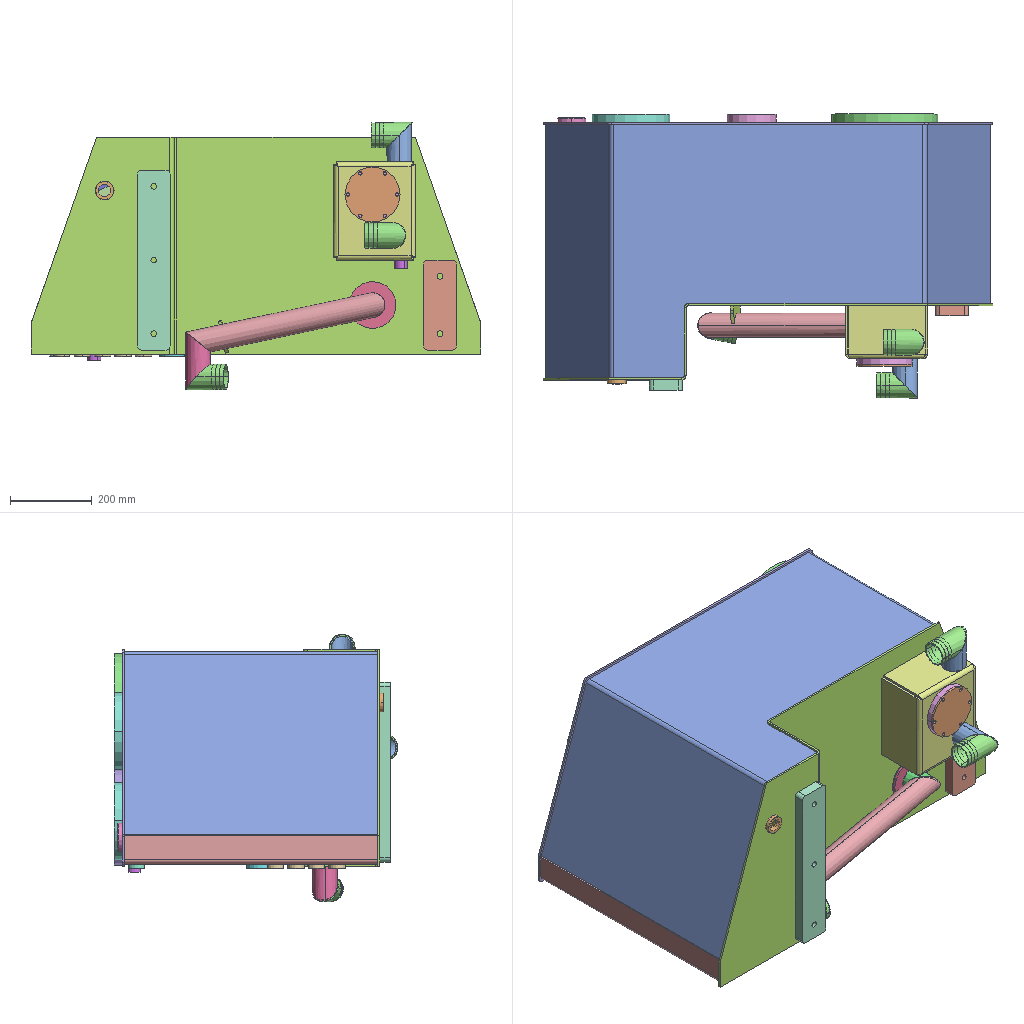Assembly | SolidWorks | 33 different items | 45 placed | box 1100 x 694 x 654 mm
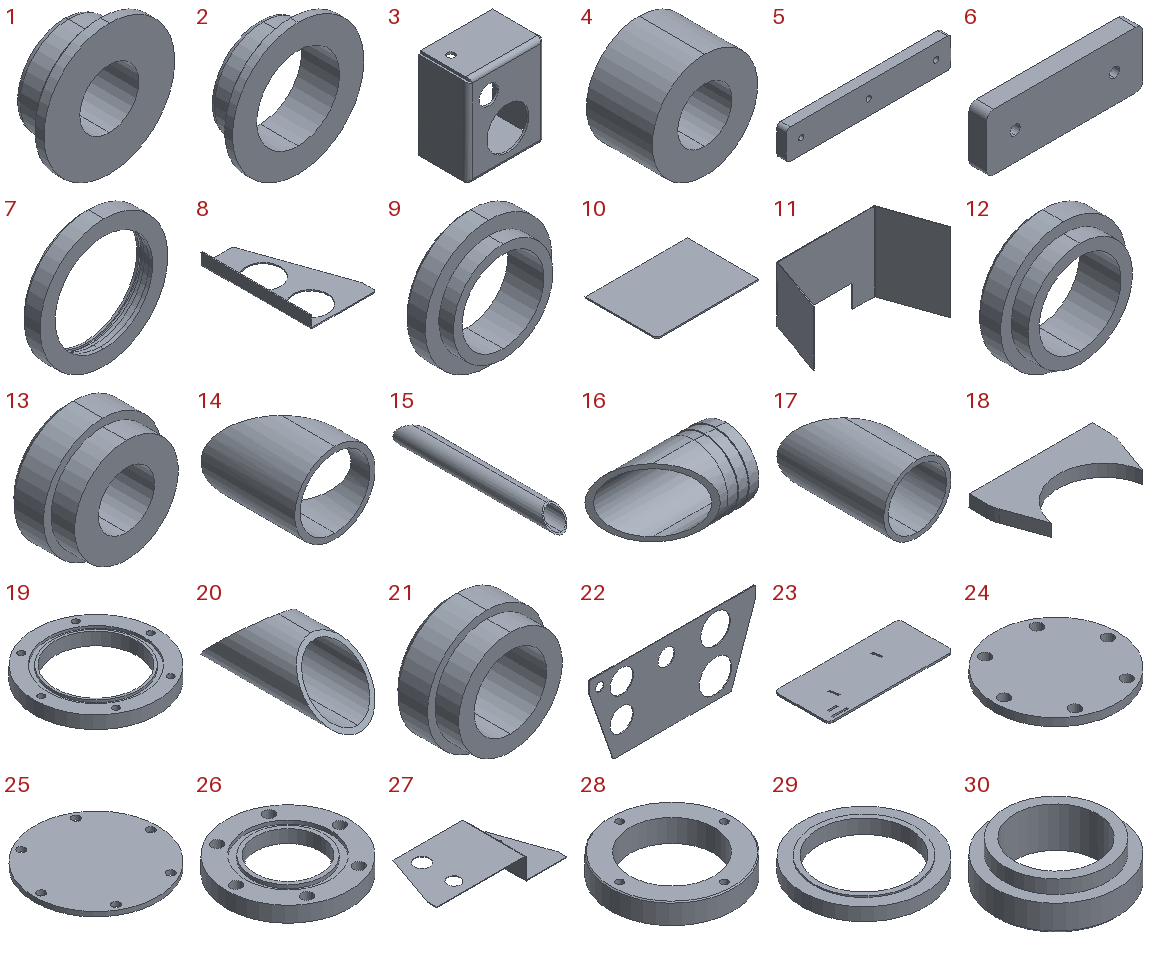Parts list (item | quantity | size | volume | features):
1 | x1 | 115 x 39 x 115 mm | 186319 mm3 | features Chamfer 1, Revolution 1
2 | x1 | 135 x 39 x 135 mm | 150743 mm3 | features Chamfer 1, Revolution 1
3 | x1 | 200 x 130 x 240 mm | 676018 mm3 | features ICE 5, Cut 1, EdgeFlange 1, FlatPattern 1, SMBaseFlange 1, SheetMetal 1, UnFold 1
4 | x2 | 32 x 20 x 32 mm | 11591 mm3 | features Chamfer 1, Extrusion 1, HoleWzd 1
5 | x1 | 440 x 25 x 80 mm | 866309 mm3 | features Fillet 1, FlatPattern 1, HoleWzd 1, LPattern 1, SMBaseFlange 1, SheetMetal 1
6 | x1 | 220 x 25 x 80 mm | 430157 mm3 | features Fillet 1, FlatPattern 1, HoleWzd 1, LPattern 1, SMBaseFlange 1, SheetMetal 1
7 | x2 | 170 x 26 x 170 mm | 194901 mm3 | features Revolution 1
8 | x1 | 305 x 510 x 58 mm | 526681 mm3 | features EdgeFlange 1, FlatPattern 1, ICE 1, SMBaseFlange 1, SheetMetal 1, UnFold 1
9 | x1 | 70 x 20 x 70 mm | 32594 mm3 | features Chamfer 1, HoleWzd 1, Revolution 1
10 | x2 | 400 x 280 x 5 mm | 559750 mm3 | features Chamfer 1, FlatPattern 1, ICE 1, LPattern 1, SMBaseFlange 1, SheetMetal 1
11 | x1 | 1088 x 449.658 x 620 mm | 4342657 mm3 | features Fillet 2, Cut 1, FlatPattern 1, SMBaseFlange 1, SheetMetal 1, UnFold 1
12 | x1 | 60 x 20 x 60 mm | 25069 mm3 | features Chamfer 1, HoleWzd 1, Revolution 1
13 | x6 | 40 x 20 x 40 mm | 16863 mm3 | features Chamfer 1, HoleWzd 1, Revolution 1
14 | x1 | 60 x 70 x 60 mm | 28148 mm3 | features Extrusion 1, ICE 1
15 | x1 | 60 x 490 x 60 mm | 306614 mm3 | features ICE 2, Extrusion 1
16 | x3 | 100 x 63 x 63 mm | 47848 mm3 | features ICE 1, Revolution 1
17 | x2 | 60 x 95 x 60 mm | 45740 mm3 | features Extrusion 1, ICE 1
18 | x1 | 80 x 43.435 x 8 mm | 16306 mm3 | features Fillet 1, FlatPattern 1, SMBaseFlange 1, SheetMetal 1
19 | x1 | 135 x 135 x 14 mm | 104256 mm3 | features ICE 2, CirPattern 1, FlatPattern 1, HoleWzd 1, SMBaseFlange 1, SheetMetal 1
20 | x1 | 60 x 140 x 60 mm | 60313 mm3 | features BaseBody 1
21 | x1 | 40 x 20 x 40 mm | 13105 mm3 | features Chamfer 1, HoleWzd 1, Revolution 1
22 | x1 | 1100 x 5 x 530 mm | 1971755 mm3 | features Fillet 1, FlatPattern 1, ICE 1, SMBaseFlange 1, SheetMetal 1
23 | x1 | 550 x 240 x 8 mm | 1041413 mm3 | features FlatPattern 1, SMBaseFlange 1, SheetMetal 1
24 | x1 | 95 x 95 x 6 mm | 40486 mm3 | features FlatPattern 1, SMBaseFlange 1, SheetMetal 1
25 | x1 | 135 x 135 x 5 mm | 69867 mm3 | features CirPattern 1, FlatPattern 1, ICE 1, SMBaseFlange 1, SheetMetal 1
26 | x1 | 95 x 95 x 12 mm | 53096 mm3 | features ICE 2, CirPattern 1, FlatPattern 1, HoleWzd 1, SMBaseFlange 1, SheetMetal 1
27 | x1 | 1100 x 530 x 187 mm | 2899151 mm3 | features Cut 2, EdgeFlange 2, ICE 2, FlatPattern 1, SMBaseFlange 1, SheetMetal 1, UnFold 1
28 | x1 | 120 x 120 x 22 mm | 125864 mm3 | features Chamfer 1, CirPattern 1, FlatPattern 1, HoleWzd 1, ICE 1, SMBaseFlange 1, SheetMetal 1
29 | x2 | 190 x 190 x 22 mm | 258295 mm3 | features ICE 2, 3DProfileFeature 1, CirPattern 1, FlatPattern 1, HoleWzd 1, SMBaseFlange 1, SheetMetal 1
30 | x1 | 46 x 46 x 15 mm | 11079 mm3 | features ICE 3, Chamfer 1, Extrusion 1, HoleWzd 1
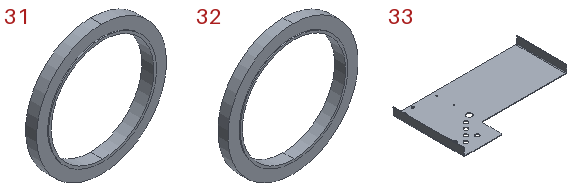31 | x1 | 235 x 22 x 235 mm | 321081 mm3 | features CirPattern 1, FlatPattern 1, HoleWzd 1, ICE 1, SMBaseFlange 1, SheetMetal 1
32 | x1 | 260 x 22 x 260 mm | 392882 mm3 | features CirPattern 1, FlatPattern 1, HoleWzd 1, ICE 1, SMBaseFlange 1, SheetMetal 1
33 | x1 | 1090 x 620 x 70 mm | 2975093 mm3 | features Cut 3, Fillet 2, EdgeFlange 1, FlatPattern 1, ICE 1, SMBaseFlange 1, SheetMetal 1, UnFold 1
Mates (type | each side: item.copy, entity, surface, feature):
Coincident | 33.1 face plane Edge-Flange1 | 11.1 face plane Base-Flange1
Coincident | 33.1 face plane Cut-Extrude1 | 27.1 face plane Base-Flange1
Parallel | 33.1 face plane Edge-Flange1 | 31.1 plane
Parallel | 32.1 plane | 33.1 face plane Edge-Flange1
Concentric | 27.1 face cylinder Cut-Extrude4 | 2.1 face cylinder Revolve1
Coincident | 27.1 face plane Base-Flange1 | 2.1 face plane Revolve1
Coincident | 27.1 face plane Base-Flange1 | 3.1 face plane Edge-Flange1
DistanceDim | 3.1 face plane Edge-Flange1 | 27.1 face plane Base-Flange1 | 2 times
Coincident | 27.1 face plane Edge-Flange2 | 5.1 face plane Base-Flange1
DistanceDim | 5.1 face plane Base-Flange1 | 27.1 face plane Edge-Flange2
DistanceDim | 5.1 face plane Base-Flange1 | 27.1 face plane Edge-Flange1
Coincident | 27.1 face plane Base-Flange1 | 6.1 face plane Base-Flange1
DistanceDim | 6.1 face plane Base-Flange1 | 27.1 face plane Base-Flange1 | 2 times
Parallel | 33.1 face plane Base-Flange1 | 28.1 plane
Coincident | 27.1 face plane Edge-Flange2 | 30.1 face plane Boss-Extrude2
Concentric | 27.1 face cylinder Cut-Extrude7 | 30.1 face cylinder Boss-Extrude3
Coincident | 33.1 face plane Base-Flange1 | 8.1 face plane Base-Flange1
Coincident | 33.1 face plane Edge-Flange1 | 8.1 face plane Base-Flange1
Coincident | 8.1 face plane Base-Flange1 | 7.1 face plane Revolve1
Concentric | 8.1 face cylinder Cut-Extrude1 | 7.1 face cylinder Revolve1
Coincident | 8.1 face plane Base-Flange1 | 7.2 face plane Revolve1
Concentric | 8.1 face cylinder Cut-Extrude1 | 7.2 face cylinder Revolve1
Coincident | 27.1 face plane Base-Flange1 | 10.1 face plane Base-Flange1
DistanceDim | 10.1 face plane Base-Flange1 | 33.1 face plane Edge-Flange1
Coincident | 33.1 face plane Base-Flange1 | 10.1 face plane Base-Flange1
Concentric | 33.1 face cylinder Cut-Extrude2 | 12.1 face cylinder Revolve1
Coincident | 33.1 face plane Base-Flange1 | 12.1 face plane Revolve1
Concentric | 33.1 face cylinder Cut-Extrude2 | 13.1 face cylinder Revolve1
Coincident | 33.1 face plane Base-Flange1 | 13.1 face plane Revolve1
Concentric | 33.1 face cylinder Cut-Extrude2 | 13.2 face cylinder Revolve1
Concentric | 33.1 face cylinder Cut-Extrude2 | 13.3 face cylinder Revolve1
Concentric | 33.1 face cylinder Cut-Extrude2 | 13.4 face cylinder Revolve1
Coincident | 33.1 face plane Base-Flange1 | 13.4 face plane Revolve1
Coincident | 33.1 face plane Base-Flange1 | 13.3 face plane Revolve1
Coincident | 33.1 face plane Base-Flange1 | 13.2 face plane Revolve1
Coincident | 3.1 face plane Edge-Flange1 | 4.1 face plane Boss-Extrude1
Concentric | 3.1 face cylinder Cut-Extrude2 | 4.1 face cylinder Boss-Extrude1
Coincident | 33.1 face plane Base-Flange1 | 4.2 face plane Boss-Extrude1
Concentric | 33.1 face cylinder Cut-Extrude3 | 4.2 face cylinder Boss-Extrude1
Coincident | 1.1 face plane Revolve1 | 14.1 face plane Boss-Extrude1
Coincident | 14.1 face plane Cut-Extrude1 | 15.1 face plane Cut-Extrude1
Coincident | 14.1 plane | 15.1 plane
DistanceDim | 15.1 plane | 1.1 face plane Revolve1
Coincident | 3.1 face plane Edge-Flange1 | 17.1 face plane Boss-Extrude1
Concentric | 3.1 face cylinder Cut-Extrude3 | 17.1 face cylinder Boss-Extrude1
Parallel | 3.1 face plane Base-Flange1 | 17.1 plane
Coincident | 3.1 face plane Base-Flange1 | 17.2 face plane Boss-Extrude1
Concentric | 3.1 face cylinder Cut-Extrude4 | 17.2 face cylinder Boss-Extrude1
Parallel | 3.1 face plane Edge-Flange1 | 17.2 plane
Coincident | 27.1 face plane Base-Flange1 | 18.1 face plane Base-Flange1
Concentric | 15.1 face cylinder Boss-Extrude1 | 18.1 face cylinder Base-Flange1
Concentric | 3.1 face cylinder Cut-Extrude6 | 19.1 face cylinder Base-Flange1
Coincident | 3.1 face plane Base-Flange1 | 19.1 face plane Base-Flange1
Parallel | 3.1 face plane Edge-Flange1 | 19.1 plane
Concentric | 27.1 face cylinder Cut-Extrude4 | 1.1 face cylinder Revolve1
Coincident | 13.4 face plane Revolve1 | 13.5 face plane Revolve1
Concentric | 33.1 face cylinder Cut-Extrude4 | 13.5 face cylinder Revolve1
Coincident | 13.4 face plane Revolve1 | 13.6 face plane Revolve1
Concentric | 33.1 face cylinder Cut-Extrude4 | 13.6 face cylinder Revolve1
Coincident | 11.1 face plane Base-Flange1 | 10.2 face plane Base-Flange1
DistanceDim | 10.2 face plane Base-Flange1 | 33.1 face plane Edge-Flange1
Coincident | 27.1 face plane Base-Flange1 | 10.2 face plane Base-Flange1
Coincident | 33.1 face plane Base-Flange1 | 21.1 face plane Revolve1
Concentric | 33.1 face cylinder Cut-Extrude3 | 21.1 face cylinder Revolve1
Coincident | 19.1 face plane Base-Flange1 | 25.1 face plane Base-Flange1
Concentric | 19.1 face cylinder Base-Flange1 | 25.1 face cylinder Base-Flange1
Concentric | 19.1 face cylinder CirPattern1 | 25.1 face cylinder CirPattern1
DistanceDim | 33.1 face plane Edge-Flange1 | 27.1 face plane Edge-Flange2
Coincident | 11.1 face plane Cut-Extrude2 | 27.1 face plane Edge-Flange1
DistanceDim | 11.1 face plane Base-Flange1 | 27.1 face plane Edge-Flange1
Coincident | 11.1 face plane Base-Flange1 | 22.1 face plane Base-Flange1
DistanceDim | 33.1 face plane Base-Flange1 | 22.1 face plane Base-Flange1
DistanceDim | 33.1 face plane Edge-Flange1 | 22.1 face plane Base-Flange1
Coincident | 17.1 face plane Cut-Extrude1 | 16.1 face plane Cut-Extrude1
DistanceDim | 16.1 face cylinder Revolve1 | 3.1 face plane Base-Flange1
DistanceDim | 3.1 face plane Edge-Flange1 | 16.1 face plane Revolve1
Coincident | 17.2 face plane Cut-Extrude1 | 16.2 face plane Cut-Extrude1
DistanceDim | 16.2 face cylinder Revolve1 | 3.1 face plane Edge-Flange1
DistanceDim | 16.2 face cylinder Revolve1 | 3.1 face plane Base-Flange1
Coincident | 27.1 face plane Base-Flange1 | 22.1 face plane Base-Flange1
Coincident | 15.1 face plane Cut-Extrude2 | 20.1 face plane Input1
DistanceDim | 20.1 face cylinder Input1 | 27.1 face plane Base-Flange1
DistanceDim | 20.1 face cylinder Input1 | 27.1 face plane Edge-Flange1
Coincident | 20.1 face plane Input1 | 16.3 face plane Cut-Extrude1
PlanarAngleDim | 16.3 face plane Revolve1 | 27.1 face plane Edge-Flange1
Concentric | 1.1 face cylinder Revolve1 | 14.1 face cylinder Boss-Extrude1